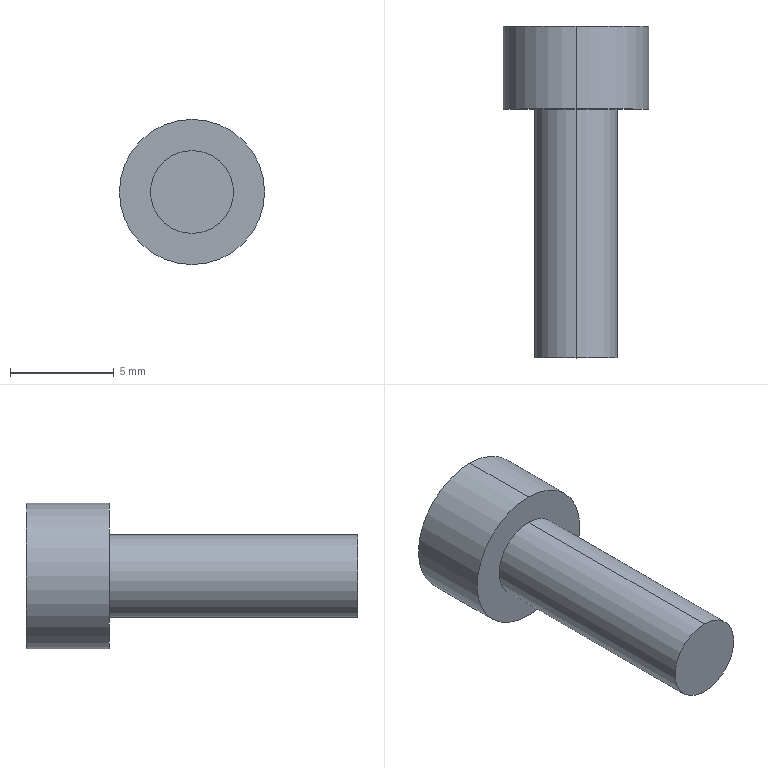Part | STEP file | NEZI-L_E-LMPJC30L35-14-15-LK5 | 1 solid | 14 faces | box 7 x 16 x 7 mm | volume 288.41 mm3 | plane 10 | cylinder 4 | commonest cylinder face diameters 4 x2 7 x2
STEP:
#1=CARTESIAN_POINT('',(0.,0.,0.));
#2=DIRECTION('',(0.,0.,1.));
#3=DIRECTION('',(1.,0.,0.));
#4=AXIS2_PLACEMENT_3D('',#1,#2,#3);
#5=CARTESIAN_POINT('',(0.,-12.,-2.));
#6=VERTEX_POINT('',#5);
#7=CARTESIAN_POINT('',(0.,-12.,2.));
#8=VERTEX_POINT('',#7);
#9=CARTESIAN_POINT('',(0.,-12.,0.));
#10=DIRECTION('',(0.,-1.,0.));
#11=DIRECTION('',(0.,0.,-1.));
#12=AXIS2_PLACEMENT_3D('',#9,#10,#11);
#13=CIRCLE('',#12,2.);
#14=CARTESIAN_POINT('',(0.,-12.,0.));
#15=DIRECTION('',(0.,1.,0.));
#16=DIRECTION('',(0.,0.,1.));
#17=AXIS2_PLACEMENT_3D('',#14,#15,#16);
#18=CYLINDRICAL_SURFACE('',#17,2.);
#19=CARTESIAN_POINT('',(3.142,0.));
#20=DIRECTION('',(-1.,0.));
#21=VECTOR('',#20,1.);
#22=LINE('',#19,#21);
#23=(GEOMETRIC_REPRESENTATION_CONTEXT(2)PARAMETRIC_REPRESENTATION_CONTEXT()REPRESENTATION_CONTEXT('',''));
#24=DEFINITIONAL_REPRESENTATION('',(#22),#23);
#25=PCURVE('',#18,#24);
#26=CARTESIAN_POINT('',(0.,-12.,0.));
#27=DIRECTION('',(0.,-1.,0.));
#28=DIRECTION('',(0.,0.,-1.));
#29=AXIS2_PLACEMENT_3D('',#26,#27,#28);
#30=PLANE('',#29);
#31=CARTESIAN_POINT('',(0.,0.));
#32=DIRECTION('',(1.,0.));
#33=AXIS2_PLACEMENT_2D('',#31,#32);
#34=CIRCLE('',#33,2.);
#35=(GEOMETRIC_REPRESENTATION_CONTEXT(2)PARAMETRIC_REPRESENTATION_CONTEXT()REPRESENTATION_CONTEXT('',''));
#36=DEFINITIONAL_REPRESENTATION('',(#34),#35);
#37=PCURVE('',#30,#36);
#38=SURFACE_CURVE('',#13,(#25,#37),.PCURVE_S1.);
#39=EDGE_CURVE('',#6,#8,#38,.T.);
#40=ORIENTED_EDGE('',*,*,#39,.F.);
#41=CARTESIAN_POINT('',(0.,0.,-2.));
#42=VERTEX_POINT('',#41);
#43=CARTESIAN_POINT('',(0.,-12.,-2.));
#44=DIRECTION('',(0.,1.,0.));
#45=VECTOR('',#44,1.);
#46=LINE('',#43,#45);
#47=CARTESIAN_POINT('',(3.142,0.));
#48=DIRECTION('',(0.,1.));
#49=VECTOR('',#48,1.);
#50=LINE('',#47,#49);
#51=(GEOMETRIC_REPRESENTATION_CONTEXT(2)PARAMETRIC_REPRESENTATION_CONTEXT()REPRESENTATION_CONTEXT('',''));
#52=DEFINITIONAL_REPRESENTATION('',(#50),#51);
#53=PCURVE('',#18,#52);
#54=CARTESIAN_POINT('',(0.,-12.,0.));
#55=DIRECTION('',(0.,1.,0.));
#56=DIRECTION('',(0.,0.,1.));
#57=AXIS2_PLACEMENT_3D('',#54,#55,#56);
#58=CYLINDRICAL_SURFACE('',#57,2.);
#59=CARTESIAN_POINT('',(3.142,0.));
#60=DIRECTION('',(0.,1.));
#61=VECTOR('',#60,1.);
#62=LINE('',#59,#61);
#63=(GEOMETRIC_REPRESENTATION_CONTEXT(2)PARAMETRIC_REPRESENTATION_CONTEXT()REPRESENTATION_CONTEXT('',''));
#64=DEFINITIONAL_REPRESENTATION('',(#62),#63);
#65=PCURVE('',#58,#64);
#66=SURFACE_CURVE('',#46,(#53,#65),.PCURVE_S1.);
#67=EDGE_CURVE('',#6,#42,#66,.T.);
#68=ORIENTED_EDGE('',*,*,#67,.T.);
#69=CARTESIAN_POINT('',(0.,0.,2.));
#70=VERTEX_POINT('',#69);
#71=CARTESIAN_POINT('',(0.,0.,0.));
#72=DIRECTION('',(0.,-1.,0.));
#73=DIRECTION('',(0.,0.,1.));
#74=AXIS2_PLACEMENT_3D('',#71,#72,#73);
#75=CIRCLE('',#74,2.);
#76=CARTESIAN_POINT('',(6.283,12.));
#77=DIRECTION('',(-1.,0.));
#78=VECTOR('',#77,1.);
#79=LINE('',#76,#78);
#80=(GEOMETRIC_REPRESENTATION_CONTEXT(2)PARAMETRIC_REPRESENTATION_CONTEXT()REPRESENTATION_CONTEXT('',''));
#81=DEFINITIONAL_REPRESENTATION('',(#79),#80);
#82=PCURVE('',#18,#81);
#83=CARTESIAN_POINT('',(0.,0.,0.));
#84=DIRECTION('',(0.,1.,0.));
#85=DIRECTION('',(0.,0.,1.));
#86=AXIS2_PLACEMENT_3D('',#83,#84,#85);
#87=PLANE('',#86);
#88=CARTESIAN_POINT('',(2.,0.));
#89=CARTESIAN_POINT('',(2.,-3.464));
#90=CARTESIAN_POINT('',(-1.,-1.732));
#91=CARTESIAN_POINT('',(-4.,0.));
#92=CARTESIAN_POINT('',(-1.,1.732));
#93=CARTESIAN_POINT('',(2.,3.464));
#94=CARTESIAN_POINT('',(2.,0.));
#95=(BOUNDED_CURVE()B_SPLINE_CURVE(2,(#88,#89,#90,#91,#92,#93,#94),.UNSPECIFIED.,.T.,.F.)B_SPLINE_CURVE_WITH_KNOTS((1,2,2,2,2,1),(-2.094,0.,2.094,4.189,6.283,8.378),.UNSPECIFIED.)CURVE()GEOMETRIC_REPRESENTATION_ITEM()RATIONAL_B_SPLINE_CURVE((1.,0.5,1.,0.5,1.,0.5,1.))REPRESENTATION_ITEM(''));
#96=(GEOMETRIC_REPRESENTATION_CONTEXT(2)PARAMETRIC_REPRESENTATION_CONTEXT()REPRESENTATION_CONTEXT('',''));
#97=DEFINITIONAL_REPRESENTATION('',(#95),#96);
#98=PCURVE('',#87,#97);
#99=SURFACE_CURVE('',#75,(#82,#98),.PCURVE_S1.);
#100=EDGE_CURVE('',#42,#70,#99,.T.);
#101=ORIENTED_EDGE('',*,*,#100,.T.);
#102=CARTESIAN_POINT('',(0.,-12.,2.));
#103=DIRECTION('',(0.,1.,0.));
#104=VECTOR('',#103,1.);
#105=LINE('',#102,#104);
#106=CARTESIAN_POINT('',(0.,0.));
#107=DIRECTION('',(0.,1.));
#108=VECTOR('',#107,1.);
#109=LINE('',#106,#108);
#110=(GEOMETRIC_REPRESENTATION_CONTEXT(2)PARAMETRIC_REPRESENTATION_CONTEXT()REPRESENTATION_CONTEXT('',''));
#111=DEFINITIONAL_REPRESENTATION('',(#109),#110);
#112=PCURVE('',#18,#111);
#113=CARTESIAN_POINT('',(6.283,0.));
#114=DIRECTION('',(0.,1.));
#115=VECTOR('',#114,1.);
#116=LINE('',#113,#115);
#117=(GEOMETRIC_REPRESENTATION_CONTEXT(2)PARAMETRIC_REPRESENTATION_CONTEXT()REPRESENTATION_CONTEXT('',''));
#118=DEFINITIONAL_REPRESENTATION('',(#116),#117);
#119=PCURVE('',#58,#118);
#120=SURFACE_CURVE('',#105,(#112,#119),.PCURVE_S1.);
#121=EDGE_CURVE('',#8,#70,#120,.T.);
#122=ORIENTED_EDGE('',*,*,#121,.F.);
#123=EDGE_LOOP('',(#40,#68,#101,#122));
#124=FACE_BOUND('',#123,.T.);
#125=ADVANCED_FACE('',(#124),#18,.T.);
#126=CARTESIAN_POINT('',(0.,4.,3.5));
#127=VERTEX_POINT('',#126);
#128=CARTESIAN_POINT('',(0.,4.,-3.5));
#129=VERTEX_POINT('',#128);
#130=CARTESIAN_POINT('',(0.,4.,0.));
#131=DIRECTION('',(0.,1.,0.));
#132=DIRECTION('',(0.,0.,1.));
#133=AXIS2_PLACEMENT_3D('',#130,#131,#132);
#134=CIRCLE('',#133,3.5);
#135=CARTESIAN_POINT('',(0.,4.,0.));
#136=DIRECTION('',(0.,-1.,0.));
#137=DIRECTION('',(0.,0.,-1.));
#138=AXIS2_PLACEMENT_3D('',#135,#136,#137);
#139=CYLINDRICAL_SURFACE('',#138,3.5);
#140=CARTESIAN_POINT('',(3.142,0.));
#141=DIRECTION('',(-1.,0.));
#142=VECTOR('',#141,1.);
#143=LINE('',#140,#142);
#144=(GEOMETRIC_REPRESENTATION_CONTEXT(2)PARAMETRIC_REPRESENTATION_CONTEXT()REPRESENTATION_CONTEXT('',''));
#145=DEFINITIONAL_REPRESENTATION('',(#143),#144);
#146=PCURVE('',#139,#145);
#147=CARTESIAN_POINT('',(0.,4.,0.));
#148=DIRECTION('',(0.,1.,0.));
#149=DIRECTION('',(0.,0.,1.));
#150=AXIS2_PLACEMENT_3D('',#147,#148,#149);
#151=PLANE('',#150);
#152=CARTESIAN_POINT('',(0.,0.));
#153=DIRECTION('',(1.,0.));
#154=AXIS2_PLACEMENT_2D('',#152,#153);
#155=CIRCLE('',#154,3.5);
#156=(GEOMETRIC_REPRESENTATION_CONTEXT(2)PARAMETRIC_REPRESENTATION_CONTEXT()REPRESENTATION_CONTEXT('',''));
#157=DEFINITIONAL_REPRESENTATION('',(#155),#156);
#158=PCURVE('',#151,#157);
#159=SURFACE_CURVE('',#134,(#146,#158),.PCURVE_S1.);
#160=EDGE_CURVE('',#127,#129,#159,.T.);
#161=ORIENTED_EDGE('',*,*,#160,.F.);
#162=CARTESIAN_POINT('',(0.,0.,3.5));
#163=VERTEX_POINT('',#162);
#164=CARTESIAN_POINT('',(0.,4.,3.5));
#165=DIRECTION('',(0.,-1.,0.));
#166=VECTOR('',#165,1.);
#167=LINE('',#164,#166);
#168=CARTESIAN_POINT('',(3.142,0.));
#169=DIRECTION('',(0.,1.));
#170=VECTOR('',#169,1.);
#171=LINE('',#168,#170);
#172=(GEOMETRIC_REPRESENTATION_CONTEXT(2)PARAMETRIC_REPRESENTATION_CONTEXT()REPRESENTATION_CONTEXT('',''));
#173=DEFINITIONAL_REPRESENTATION('',(#171),#172);
#174=PCURVE('',#139,#173);
#175=CARTESIAN_POINT('',(0.,4.,0.));
#176=DIRECTION('',(0.,-1.,0.));
#177=DIRECTION('',(0.,0.,-1.));
#178=AXIS2_PLACEMENT_3D('',#175,#176,#177);
#179=CYLINDRICAL_SURFACE('',#178,3.5);
#180=CARTESIAN_POINT('',(3.142,0.));
#181=DIRECTION('',(0.,1.));
#182=VECTOR('',#181,1.);
#183=LINE('',#180,#182);
#184=(GEOMETRIC_REPRESENTATION_CONTEXT(2)PARAMETRIC_REPRESENTATION_CONTEXT()REPRESENTATION_CONTEXT('',''));
#185=DEFINITIONAL_REPRESENTATION('',(#183),#184);
#186=PCURVE('',#179,#185);
#187=SURFACE_CURVE('',#167,(#174,#186),.PCURVE_S1.);
#188=EDGE_CURVE('',#127,#163,#187,.T.);
#189=ORIENTED_EDGE('',*,*,#188,.T.);
#190=CARTESIAN_POINT('',(0.,0.,-3.5));
#191=VERTEX_POINT('',#190);
#192=CARTESIAN_POINT('',(0.,0.,0.));
#193=DIRECTION('',(0.,1.,0.));
#194=DIRECTION('',(0.,0.,1.));
#195=AXIS2_PLACEMENT_3D('',#192,#193,#194);
#196=CIRCLE('',#195,3.5);
#197=CARTESIAN_POINT('',(3.142,4.));
#198=DIRECTION('',(-1.,0.));
#199=VECTOR('',#198,1.);
#200=LINE('',#197,#199);
#201=(GEOMETRIC_REPRESENTATION_CONTEXT(2)PARAMETRIC_REPRESENTATION_CONTEXT()REPRESENTATION_CONTEXT('',''));
#202=DEFINITIONAL_REPRESENTATION('',(#200),#201);
#203=PCURVE('',#139,#202);
#204=CARTESIAN_POINT('',(0.,0.));
#205=DIRECTION('',(1.,0.));
#206=AXIS2_PLACEMENT_2D('',#204,#205);
#207=CIRCLE('',#206,3.5);
#208=(GEOMETRIC_REPRESENTATION_CONTEXT(2)PARAMETRIC_REPRESENTATION_CONTEXT()REPRESENTATION_CONTEXT('',''));
#209=DEFINITIONAL_REPRESENTATION('',(#207),#208);
#210=PCURVE('',#87,#209);
#211=SURFACE_CURVE('',#196,(#203,#210),.PCURVE_S1.);
#212=EDGE_CURVE('',#163,#191,#211,.T.);
#213=ORIENTED_EDGE('',*,*,#212,.T.);
#214=CARTESIAN_POINT('',(0.,4.,-3.5));
#215=DIRECTION('',(0.,-1.,0.));
#216=VECTOR('',#215,1.);
#217=LINE('',#214,#216);
#218=CARTESIAN_POINT('',(0.,0.));
#219=DIRECTION('',(0.,1.));
#220=VECTOR('',#219,1.);
#221=LINE('',#218,#220);
#222=(GEOMETRIC_REPRESENTATION_CONTEXT(2)PARAMETRIC_REPRESENTATION_CONTEXT()REPRESENTATION_CONTEXT('',''));
#223=DEFINITIONAL_REPRESENTATION('',(#221),#222);
#224=PCURVE('',#139,#223);
#225=CARTESIAN_POINT('',(6.283,0.));
#226=DIRECTION('',(0.,1.));
#227=VECTOR('',#226,1.);
#228=LINE('',#225,#227);
#229=(GEOMETRIC_REPRESENTATION_CONTEXT(2)PARAMETRIC_REPRESENTATION_CONTEXT()REPRESENTATION_CONTEXT('',''));
#230=DEFINITIONAL_REPRESENTATION('',(#228),#229);
#231=PCURVE('',#179,#230);
#232=SURFACE_CURVE('',#217,(#224,#231),.PCURVE_S1.);
#233=EDGE_CURVE('',#129,#191,#232,.T.);
#234=ORIENTED_EDGE('',*,*,#233,.F.);
#235=EDGE_LOOP('',(#161,#189,#213,#234));
#236=FACE_BOUND('',#235,.T.);
#237=ADVANCED_FACE('',(#236),#139,.T.);
#238=ORIENTED_EDGE('',*,*,#188,.F.);
#239=CARTESIAN_POINT('',(0.,4.,0.));
#240=DIRECTION('',(0.,1.,0.));
#241=DIRECTION('',(0.,0.,1.));
#242=AXIS2_PLACEMENT_3D('',#239,#240,#241);
#243=CIRCLE('',#242,3.5);
#244=CARTESIAN_POINT('',(9.425,0.));
#245=DIRECTION('',(-1.,0.));
#246=VECTOR('',#245,1.);
#247=LINE('',#244,#246);
#248=(GEOMETRIC_REPRESENTATION_CONTEXT(2)PARAMETRIC_REPRESENTATION_CONTEXT()REPRESENTATION_CONTEXT('',''));
#249=DEFINITIONAL_REPRESENTATION('',(#247),#248);
#250=PCURVE('',#179,#249);
#251=CARTESIAN_POINT('',(0.,0.));
#252=DIRECTION('',(1.,0.));
#253=AXIS2_PLACEMENT_2D('',#251,#252);
#254=CIRCLE('',#253,3.5);
#255=(GEOMETRIC_REPRESENTATION_CONTEXT(2)PARAMETRIC_REPRESENTATION_CONTEXT()REPRESENTATION_CONTEXT('',''));
#256=DEFINITIONAL_REPRESENTATION('',(#254),#255);
#257=PCURVE('',#151,#256);
#258=SURFACE_CURVE('',#243,(#250,#257),.PCURVE_S1.);
#259=EDGE_CURVE('',#129,#127,#258,.T.);
#260=ORIENTED_EDGE('',*,*,#259,.F.);
#261=ORIENTED_EDGE('',*,*,#233,.T.);
#262=CARTESIAN_POINT('',(0.,0.,0.));
#263=DIRECTION('',(0.,1.,0.));
#264=DIRECTION('',(0.,0.,1.));
#265=AXIS2_PLACEMENT_3D('',#262,#263,#264);
#266=CIRCLE('',#265,3.5);
#267=CARTESIAN_POINT('',(9.425,4.));
#268=DIRECTION('',(-1.,0.));
#269=VECTOR('',#268,1.);
#270=LINE('',#267,#269);
#271=(GEOMETRIC_REPRESENTATION_CONTEXT(2)PARAMETRIC_REPRESENTATION_CONTEXT()REPRESENTATION_CONTEXT('',''));
#272=DEFINITIONAL_REPRESENTATION('',(#270),#271);
#273=PCURVE('',#179,#272);
#274=CARTESIAN_POINT('',(0.,0.));
#275=DIRECTION('',(1.,0.));
#276=AXIS2_PLACEMENT_2D('',#274,#275);
#277=CIRCLE('',#276,3.5);
#278=(GEOMETRIC_REPRESENTATION_CONTEXT(2)PARAMETRIC_REPRESENTATION_CONTEXT()REPRESENTATION_CONTEXT('',''));
#279=DEFINITIONAL_REPRESENTATION('',(#277),#278);
#280=PCURVE('',#87,#279);
#281=SURFACE_CURVE('',#266,(#273,#280),.PCURVE_S1.);
#282=EDGE_CURVE('',#191,#163,#281,.T.);
#283=ORIENTED_EDGE('',*,*,#282,.T.);
#284=EDGE_LOOP('',(#238,#260,#261,#283));
#285=FACE_BOUND('',#284,.T.);
#286=ADVANCED_FACE('',(#285),#179,.T.);
#287=CARTESIAN_POINT('',(1.535,4.,-0.8862));
#288=VERTEX_POINT('',#287);
#289=CARTESIAN_POINT('',(0.,4.,-1.772));
#290=VERTEX_POINT('',#289);
#291=CARTESIAN_POINT('',(1.535,4.,-0.8862));
#292=DIRECTION('',(-0.866,0.,-0.5));
#293=VECTOR('',#292,1.);
#294=LINE('',#291,#293);
#295=CARTESIAN_POINT('',(-0.8862,1.535));
#296=DIRECTION('',(-0.5,-0.866));
#297=VECTOR('',#296,1.);
#298=LINE('',#295,#297);
#299=(GEOMETRIC_REPRESENTATION_CONTEXT(2)PARAMETRIC_REPRESENTATION_CONTEXT()REPRESENTATION_CONTEXT('',''));
#300=DEFINITIONAL_REPRESENTATION('',(#298),#299);
#301=PCURVE('',#151,#300);
#302=CARTESIAN_POINT('',(1.535,2.,-0.8862));
#303=DIRECTION('',(0.5,0.,-0.866));
#304=DIRECTION('',(-0.866,0.,-0.5));
#305=AXIS2_PLACEMENT_3D('',#302,#303,#304);
#306=PLANE('',#305);
#307=CARTESIAN_POINT('',(0.,2.));
#308=DIRECTION('',(1.,0.));
#309=VECTOR('',#308,1.);
#310=LINE('',#307,#309);
#311=(GEOMETRIC_REPRESENTATION_CONTEXT(2)PARAMETRIC_REPRESENTATION_CONTEXT()REPRESENTATION_CONTEXT('',''));
#312=DEFINITIONAL_REPRESENTATION('',(#310),#311);
#313=PCURVE('',#306,#312);
#314=SURFACE_CURVE('',#294,(#301,#313),.PCURVE_S1.);
#315=EDGE_CURVE('',#288,#290,#314,.T.);
#316=ORIENTED_EDGE('',*,*,#315,.F.);
#317=CARTESIAN_POINT('',(1.535,4.,0.8862));
#318=VERTEX_POINT('',#317);
#319=CARTESIAN_POINT('',(1.535,4.,0.8862));
#320=DIRECTION('',(0.,0.,-1.));
#321=VECTOR('',#320,1.);
#322=LINE('',#319,#321);
#323=CARTESIAN_POINT('',(0.8862,1.535));
#324=DIRECTION('',(-1.,0.));
#325=VECTOR('',#324,1.);
#326=LINE('',#323,#325);
#327=(GEOMETRIC_REPRESENTATION_CONTEXT(2)PARAMETRIC_REPRESENTATION_CONTEXT()REPRESENTATION_CONTEXT('',''));
#328=DEFINITIONAL_REPRESENTATION('',(#326),#327);
#329=PCURVE('',#151,#328);
#330=CARTESIAN_POINT('',(1.535,2.,0.8862));
#331=DIRECTION('',(1.,0.,0.));
#332=DIRECTION('',(0.,0.,-1.));
#333=AXIS2_PLACEMENT_3D('',#330,#331,#332);
#334=PLANE('',#333);
#335=CARTESIAN_POINT('',(0.,2.));
#336=DIRECTION('',(1.,0.));
#337=VECTOR('',#336,1.);
#338=LINE('',#335,#337);
#339=(GEOMETRIC_REPRESENTATION_CONTEXT(2)PARAMETRIC_REPRESENTATION_CONTEXT()REPRESENTATION_CONTEXT('',''));
#340=DEFINITIONAL_REPRESENTATION('',(#338),#339);
#341=PCURVE('',#334,#340);
#342=SURFACE_CURVE('',#322,(#329,#341),.PCURVE_S1.);
#343=EDGE_CURVE('',#318,#288,#342,.T.);
#344=ORIENTED_EDGE('',*,*,#343,.F.);
#345=CARTESIAN_POINT('',(0.,4.,1.772));
#346=VERTEX_POINT('',#345);
#347=CARTESIAN_POINT('',(0.,4.,1.772));
#348=DIRECTION('',(0.866,0.,-0.5));
#349=VECTOR('',#348,1.);
#350=LINE('',#347,#349);
#351=CARTESIAN_POINT('',(1.772,0.));
#352=DIRECTION('',(-0.5,0.866));
#353=VECTOR('',#352,1.);
#354=LINE('',#351,#353);
#355=(GEOMETRIC_REPRESENTATION_CONTEXT(2)PARAMETRIC_REPRESENTATION_CONTEXT()REPRESENTATION_CONTEXT('',''));
#356=DEFINITIONAL_REPRESENTATION('',(#354),#355);
#357=PCURVE('',#151,#356);
#358=CARTESIAN_POINT('',(0.,2.,1.772));
#359=DIRECTION('',(0.5,0.,0.866));
#360=DIRECTION('',(0.866,0.,-0.5));
#361=AXIS2_PLACEMENT_3D('',#358,#359,#360);
#362=PLANE('',#361);
#363=CARTESIAN_POINT('',(0.,2.));
#364=DIRECTION('',(1.,0.));
#365=VECTOR('',#364,1.);
#366=LINE('',#363,#365);
#367=(GEOMETRIC_REPRESENTATION_CONTEXT(2)PARAMETRIC_REPRESENTATION_CONTEXT()REPRESENTATION_CONTEXT('',''));
#368=DEFINITIONAL_REPRESENTATION('',(#366),#367);
#369=PCURVE('',#362,#368);
#370=SURFACE_CURVE('',#350,(#357,#369),.PCURVE_S1.);
#371=EDGE_CURVE('',#346,#318,#370,.T.);
#372=ORIENTED_EDGE('',*,*,#371,.F.);
#373=CARTESIAN_POINT('',(-1.535,4.,0.8862));
#374=VERTEX_POINT('',#373);
#375=CARTESIAN_POINT('',(-1.535,4.,0.8862));
#376=DIRECTION('',(0.866,0.,0.5));
#377=VECTOR('',#376,1.);
#378=LINE('',#375,#377);
#379=CARTESIAN_POINT('',(0.8862,-1.535));
#380=DIRECTION('',(0.5,0.866));
#381=VECTOR('',#380,1.);
#382=LINE('',#379,#381);
#383=(GEOMETRIC_REPRESENTATION_CONTEXT(2)PARAMETRIC_REPRESENTATION_CONTEXT()REPRESENTATION_CONTEXT('',''));
#384=DEFINITIONAL_REPRESENTATION('',(#382),#383);
#385=PCURVE('',#151,#384);
#386=CARTESIAN_POINT('',(-1.535,2.,0.8862));
#387=DIRECTION('',(-0.5,0.,0.866));
#388=DIRECTION('',(0.866,0.,0.5));
#389=AXIS2_PLACEMENT_3D('',#386,#387,#388);
#390=PLANE('',#389);
#391=CARTESIAN_POINT('',(0.,2.));
#392=DIRECTION('',(1.,0.));
#393=VECTOR('',#392,1.);
#394=LINE('',#391,#393);
#395=(GEOMETRIC_REPRESENTATION_CONTEXT(2)PARAMETRIC_REPRESENTATION_CONTEXT()REPRESENTATION_CONTEXT('',''));
#396=DEFINITIONAL_REPRESENTATION('',(#394),#395);
#397=PCURVE('',#390,#396);
#398=SURFACE_CURVE('',#378,(#385,#397),.PCURVE_S1.);
#399=EDGE_CURVE('',#374,#346,#398,.T.);
#400=ORIENTED_EDGE('',*,*,#399,.F.);
#401=CARTESIAN_POINT('',(-1.535,4.,-0.8862));
#402=VERTEX_POINT('',#401);
#403=CARTESIAN_POINT('',(-1.535,4.,-0.8862));
#404=DIRECTION('',(0.,0.,1.));
#405=VECTOR('',#404,1.);
#406=LINE('',#403,#405);
#407=CARTESIAN_POINT('',(-0.8862,-1.535));
#408=DIRECTION('',(1.,0.));
#409=VECTOR('',#408,1.);
#410=LINE('',#407,#409);
#411=(GEOMETRIC_REPRESENTATION_CONTEXT(2)PARAMETRIC_REPRESENTATION_CONTEXT()REPRESENTATION_CONTEXT('',''));
#412=DEFINITIONAL_REPRESENTATION('',(#410),#411);
#413=PCURVE('',#151,#412);
#414=CARTESIAN_POINT('',(-1.535,2.,-0.8862));
#415=DIRECTION('',(-1.,0.,0.));
#416=DIRECTION('',(0.,0.,1.));
#417=AXIS2_PLACEMENT_3D('',#414,#415,#416);
#418=PLANE('',#417);
#419=CARTESIAN_POINT('',(0.,2.));
#420=DIRECTION('',(1.,0.));
#421=VECTOR('',#420,1.);
#422=LINE('',#419,#421);
#423=(GEOMETRIC_REPRESENTATION_CONTEXT(2)PARAMETRIC_REPRESENTATION_CONTEXT()REPRESENTATION_CONTEXT('',''));
#424=DEFINITIONAL_REPRESENTATION('',(#422),#423);
#425=PCURVE('',#418,#424);
#426=SURFACE_CURVE('',#406,(#413,#425),.PCURVE_S1.);
#427=EDGE_CURVE('',#402,#374,#426,.T.);
#428=ORIENTED_EDGE('',*,*,#427,.F.);
#429=CARTESIAN_POINT('',(0.,4.,-1.772));
#430=DIRECTION('',(-0.866,0.,0.5));
#431=VECTOR('',#430,1.);
#432=LINE('',#429,#431);
#433=CARTESIAN_POINT('',(-1.772,0.));
#434=DIRECTION('',(0.5,-0.866));
#435=VECTOR('',#434,1.);
#436=LINE('',#433,#435);
#437=(GEOMETRIC_REPRESENTATION_CONTEXT(2)PARAMETRIC_REPRESENTATION_CONTEXT()REPRESENTATION_CONTEXT('',''));
#438=DEFINITIONAL_REPRESENTATION('',(#436),#437);
#439=PCURVE('',#151,#438);
#440=CARTESIAN_POINT('',(0.,2.,-1.772));
#441=DIRECTION('',(-0.5,0.,-0.866));
#442=DIRECTION('',(-0.866,0.,0.5));
#443=AXIS2_PLACEMENT_3D('',#440,#441,#442);
#444=PLANE('',#443);
#445=CARTESIAN_POINT('',(0.,2.));
#446=DIRECTION('',(1.,0.));
#447=VECTOR('',#446,1.);
#448=LINE('',#445,#447);
#449=(GEOMETRIC_REPRESENTATION_CONTEXT(2)PARAMETRIC_REPRESENTATION_CONTEXT()REPRESENTATION_CONTEXT('',''));
#450=DEFINITIONAL_REPRESENTATION('',(#448),#449);
#451=PCURVE('',#444,#450);
#452=SURFACE_CURVE('',#432,(#439,#451),.PCURVE_S1.);
#453=EDGE_CURVE('',#290,#402,#452,.T.);
#454=ORIENTED_EDGE('',*,*,#453,.F.);
#455=EDGE_LOOP('',(#316,#344,#372,#400,#428,#454));
#456=FACE_BOUND('',#455,.T.);
#457=ORIENTED_EDGE('',*,*,#259,.T.);
#458=ORIENTED_EDGE('',*,*,#160,.T.);
#459=EDGE_LOOP('',(#457,#458));
#460=FACE_BOUND('',#459,.T.);
#461=ADVANCED_FACE('',(#456,#460),#151,.T.);
#462=CARTESIAN_POINT('',(0.,0.,0.));
#463=DIRECTION('',(0.,-1.,0.));
#464=DIRECTION('',(0.,0.,1.));
#465=AXIS2_PLACEMENT_3D('',#462,#463,#464);
#466=CIRCLE('',#465,2.);
#467=CARTESIAN_POINT('',(2.,0.));
#468=CARTESIAN_POINT('',(2.,-3.464));
#469=CARTESIAN_POINT('',(-1.,-1.732));
#470=CARTESIAN_POINT('',(-4.,0.));
#471=CARTESIAN_POINT('',(-1.,1.732));
#472=CARTESIAN_POINT('',(2.,3.464));
#473=CARTESIAN_POINT('',(2.,0.));
#474=(BOUNDED_CURVE()B_SPLINE_CURVE(2,(#467,#468,#469,#470,#471,#472,#473),.UNSPECIFIED.,.T.,.F.)B_SPLINE_CURVE_WITH_KNOTS((1,2,2,2,2,1),(-2.094,0.,2.094,4.189,6.283,8.378),.UNSPECIFIED.)CURVE()GEOMETRIC_REPRESENTATION_ITEM()RATIONAL_B_SPLINE_CURVE((1.,0.5,1.,0.5,1.,0.5,1.))REPRESENTATION_ITEM(''));
#475=(GEOMETRIC_REPRESENTATION_CONTEXT(2)PARAMETRIC_REPRESENTATION_CONTEXT()REPRESENTATION_CONTEXT('',''));
#476=DEFINITIONAL_REPRESENTATION('',(#474),#475);
#477=PCURVE('',#87,#476);
#478=CARTESIAN_POINT('',(6.283,12.));
#479=DIRECTION('',(-1.,0.));
#480=VECTOR('',#479,1.);
#481=LINE('',#478,#480);
#482=(GEOMETRIC_REPRESENTATION_CONTEXT(2)PARAMETRIC_REPRESENTATION_CONTEXT()REPRESENTATION_CONTEXT('',''));
#483=DEFINITIONAL_REPRESENTATION('',(#481),#482);
#484=PCURVE('',#58,#483);
#485=SURFACE_CURVE('',#466,(#477,#484),.PCURVE_S1.);
#486=EDGE_CURVE('',#70,#42,#485,.T.);
#487=ORIENTED_EDGE('',*,*,#486,.F.);
#488=ORIENTED_EDGE('',*,*,#100,.F.);
#489=EDGE_LOOP('',(#487,#488));
#490=FACE_BOUND('',#489,.T.);
#491=ORIENTED_EDGE('',*,*,#282,.F.);
#492=ORIENTED_EDGE('',*,*,#212,.F.);
#493=EDGE_LOOP('',(#491,#492));
#494=FACE_BOUND('',#493,.T.);
#495=ADVANCED_FACE('',(#490,#494),#87,.F.);
#496=ORIENTED_EDGE('',*,*,#67,.F.);
#497=CARTESIAN_POINT('',(0.,-12.,0.));
#498=DIRECTION('',(0.,-1.,0.));
#499=DIRECTION('',(0.,0.,-1.));
#500=AXIS2_PLACEMENT_3D('',#497,#498,#499);
#501=CIRCLE('',#500,2.);
#502=CARTESIAN_POINT('',(9.425,0.));
#503=DIRECTION('',(-1.,0.));
#504=VECTOR('',#503,1.);
#505=LINE('',#502,#504);
#506=(GEOMETRIC_REPRESENTATION_CONTEXT(2)PARAMETRIC_REPRESENTATION_CONTEXT()REPRESENTATION_CONTEXT('',''));
#507=DEFINITIONAL_REPRESENTATION('',(#505),#506);
#508=PCURVE('',#58,#507);
#509=CARTESIAN_POINT('',(0.,0.));
#510=DIRECTION('',(1.,0.));
#511=AXIS2_PLACEMENT_2D('',#509,#510);
#512=CIRCLE('',#511,2.);
#513=(GEOMETRIC_REPRESENTATION_CONTEXT(2)PARAMETRIC_REPRESENTATION_CONTEXT()REPRESENTATION_CONTEXT('',''));
#514=DEFINITIONAL_REPRESENTATION('',(#512),#513);
#515=PCURVE('',#30,#514);
#516=SURFACE_CURVE('',#501,(#508,#515),.PCURVE_S1.);
#517=EDGE_CURVE('',#8,#6,#516,.T.);
#518=ORIENTED_EDGE('',*,*,#517,.F.);
#519=ORIENTED_EDGE('',*,*,#121,.T.);
#520=ORIENTED_EDGE('',*,*,#486,.T.);
#521=EDGE_LOOP('',(#496,#518,#519,#520));
#522=FACE_BOUND('',#521,.T.);
#523=ADVANCED_FACE('',(#522),#58,.T.);
#524=ORIENTED_EDGE('',*,*,#517,.T.);
#525=ORIENTED_EDGE('',*,*,#39,.T.);
#526=EDGE_LOOP('',(#524,#525));
#527=FACE_BOUND('',#526,.T.);
#528=ADVANCED_FACE('',(#527),#30,.T.);
#529=ORIENTED_EDGE('',*,*,#315,.T.);
#530=CARTESIAN_POINT('',(0.,2.,-1.772));
#531=VERTEX_POINT('',#530);
#532=CARTESIAN_POINT('',(0.,2.,-1.772));
#533=DIRECTION('',(0.,1.,0.));
#534=VECTOR('',#533,1.);
#535=LINE('',#532,#534);
#536=CARTESIAN_POINT('',(1.772,0.));
#537=DIRECTION('',(0.,1.));
#538=VECTOR('',#537,1.);
#539=LINE('',#536,#538);
#540=(GEOMETRIC_REPRESENTATION_CONTEXT(2)PARAMETRIC_REPRESENTATION_CONTEXT()REPRESENTATION_CONTEXT('',''));
#541=DEFINITIONAL_REPRESENTATION('',(#539),#540);
#542=PCURVE('',#306,#541);
#543=CARTESIAN_POINT('',(0.,0.));
#544=DIRECTION('',(0.,1.));
#545=VECTOR('',#544,1.);
#546=LINE('',#543,#545);
#547=(GEOMETRIC_REPRESENTATION_CONTEXT(2)PARAMETRIC_REPRESENTATION_CONTEXT()REPRESENTATION_CONTEXT('',''));
#548=DEFINITIONAL_REPRESENTATION('',(#546),#547);
#549=PCURVE('',#444,#548);
#550=SURFACE_CURVE('',#535,(#542,#549),.PCURVE_S1.);
#551=EDGE_CURVE('',#531,#290,#550,.T.);
#552=ORIENTED_EDGE('',*,*,#551,.F.);
#553=CARTESIAN_POINT('',(1.535,2.,-0.8862));
#554=VERTEX_POINT('',#553);
#555=CARTESIAN_POINT('',(1.535,2.,-0.8862));
#556=DIRECTION('',(-0.866,0.,-0.5));
#557=VECTOR('',#556,1.);
#558=LINE('',#555,#557);
#559=CARTESIAN_POINT('',(0.,0.));
#560=DIRECTION('',(1.,0.));
#561=VECTOR('',#560,1.);
#562=LINE('',#559,#561);
#563=(GEOMETRIC_REPRESENTATION_CONTEXT(2)PARAMETRIC_REPRESENTATION_CONTEXT()REPRESENTATION_CONTEXT('',''));
#564=DEFINITIONAL_REPRESENTATION('',(#562),#563);
#565=PCURVE('',#306,#564);
#566=CARTESIAN_POINT('',(0.,2.,0.));
#567=DIRECTION('',(0.,1.,0.));
#568=DIRECTION('',(0.,0.,1.));
#569=AXIS2_PLACEMENT_3D('',#566,#567,#568);
#570=PLANE('',#569);
#571=CARTESIAN_POINT('',(-0.8862,1.535));
#572=DIRECTION('',(-0.5,-0.866));
#573=VECTOR('',#572,1.);
#574=LINE('',#571,#573);
#575=(GEOMETRIC_REPRESENTATION_CONTEXT(2)PARAMETRIC_REPRESENTATION_CONTEXT()REPRESENTATION_CONTEXT('',''));
#576=DEFINITIONAL_REPRESENTATION('',(#574),#575);
#577=PCURVE('',#570,#576);
#578=SURFACE_CURVE('',#558,(#565,#577),.PCURVE_S1.);
#579=EDGE_CURVE('',#554,#531,#578,.T.);
#580=ORIENTED_EDGE('',*,*,#579,.F.);
#581=CARTESIAN_POINT('',(1.535,2.,-0.8862));
#582=DIRECTION('',(0.,1.,0.));
#583=VECTOR('',#582,1.);
#584=LINE('',#581,#583);
#585=CARTESIAN_POINT('',(0.,0.));
#586=DIRECTION('',(0.,1.));
#587=VECTOR('',#586,1.);
#588=LINE('',#585,#587);
#589=(GEOMETRIC_REPRESENTATION_CONTEXT(2)PARAMETRIC_REPRESENTATION_CONTEXT()REPRESENTATION_CONTEXT('',''));
#590=DEFINITIONAL_REPRESENTATION('',(#588),#589);
#591=PCURVE('',#306,#590);
#592=CARTESIAN_POINT('',(1.772,0.));
#593=DIRECTION('',(0.,1.));
#594=VECTOR('',#593,1.);
#595=LINE('',#592,#594);
#596=(GEOMETRIC_REPRESENTATION_CONTEXT(2)PARAMETRIC_REPRESENTATION_CONTEXT()REPRESENTATION_CONTEXT('',''));
#597=DEFINITIONAL_REPRESENTATION('',(#595),#596);
#598=PCURVE('',#334,#597);
#599=SURFACE_CURVE('',#584,(#591,#598),.PCURVE_S1.);
#600=EDGE_CURVE('',#554,#288,#599,.T.);
#601=ORIENTED_EDGE('',*,*,#600,.T.);
#602=EDGE_LOOP('',(#529,#552,#580,#601));
#603=FACE_BOUND('',#602,.T.);
#604=ADVANCED_FACE('',(#603),#306,.F.);
#605=ORIENTED_EDGE('',*,*,#343,.T.);
#606=ORIENTED_EDGE('',*,*,#600,.F.);
#607=CARTESIAN_POINT('',(1.535,2.,0.8862));
#608=VERTEX_POINT('',#607);
#609=CARTESIAN_POINT('',(1.535,2.,0.8862));
#610=DIRECTION('',(0.,0.,-1.));
#611=VECTOR('',#610,1.);
#612=LINE('',#609,#611);
#613=CARTESIAN_POINT('',(0.,0.));
#614=DIRECTION('',(1.,0.));
#615=VECTOR('',#614,1.);
#616=LINE('',#613,#615);
#617=(GEOMETRIC_REPRESENTATION_CONTEXT(2)PARAMETRIC_REPRESENTATION_CONTEXT()REPRESENTATION_CONTEXT('',''));
#618=DEFINITIONAL_REPRESENTATION('',(#616),#617);
#619=PCURVE('',#334,#618);
#620=CARTESIAN_POINT('',(0.8862,1.535));
#621=DIRECTION('',(-1.,0.));
#622=VECTOR('',#621,1.);
#623=LINE('',#620,#622);
#624=(GEOMETRIC_REPRESENTATION_CONTEXT(2)PARAMETRIC_REPRESENTATION_CONTEXT()REPRESENTATION_CONTEXT('',''));
#625=DEFINITIONAL_REPRESENTATION('',(#623),#624);
#626=PCURVE('',#570,#625);
#627=SURFACE_CURVE('',#612,(#619,#626),.PCURVE_S1.);
#628=EDGE_CURVE('',#608,#554,#627,.T.);
#629=ORIENTED_EDGE('',*,*,#628,.F.);
#630=CARTESIAN_POINT('',(1.535,2.,0.8862));
#631=DIRECTION('',(0.,1.,0.));
#632=VECTOR('',#631,1.);
#633=LINE('',#630,#632);
#634=CARTESIAN_POINT('',(0.,0.));
#635=DIRECTION('',(0.,1.));
#636=VECTOR('',#635,1.);
#637=LINE('',#634,#636);
#638=(GEOMETRIC_REPRESENTATION_CONTEXT(2)PARAMETRIC_REPRESENTATION_CONTEXT()REPRESENTATION_CONTEXT('',''));
#639=DEFINITIONAL_REPRESENTATION('',(#637),#638);
#640=PCURVE('',#334,#639);
#641=CARTESIAN_POINT('',(1.772,0.));
#642=DIRECTION('',(0.,1.));
#643=VECTOR('',#642,1.);
#644=LINE('',#641,#643);
#645=(GEOMETRIC_REPRESENTATION_CONTEXT(2)PARAMETRIC_REPRESENTATION_CONTEXT()REPRESENTATION_CONTEXT('',''));
#646=DEFINITIONAL_REPRESENTATION('',(#644),#645);
#647=PCURVE('',#362,#646);
#648=SURFACE_CURVE('',#633,(#640,#647),.PCURVE_S1.);
#649=EDGE_CURVE('',#608,#318,#648,.T.);
#650=ORIENTED_EDGE('',*,*,#649,.T.);
#651=EDGE_LOOP('',(#605,#606,#629,#650));
#652=FACE_BOUND('',#651,.T.);
#653=ADVANCED_FACE('',(#652),#334,.F.);
#654=ORIENTED_EDGE('',*,*,#371,.T.);
#655=ORIENTED_EDGE('',*,*,#649,.F.);
#656=CARTESIAN_POINT('',(0.,2.,1.772));
#657=VERTEX_POINT('',#656);
#658=CARTESIAN_POINT('',(0.,2.,1.772));
#659=DIRECTION('',(0.866,0.,-0.5));
#660=VECTOR('',#659,1.);
#661=LINE('',#658,#660);
#662=CARTESIAN_POINT('',(0.,0.));
#663=DIRECTION('',(1.,0.));
#664=VECTOR('',#663,1.);
#665=LINE('',#662,#664);
#666=(GEOMETRIC_REPRESENTATION_CONTEXT(2)PARAMETRIC_REPRESENTATION_CONTEXT()REPRESENTATION_CONTEXT('',''));
#667=DEFINITIONAL_REPRESENTATION('',(#665),#666);
#668=PCURVE('',#362,#667);
#669=CARTESIAN_POINT('',(1.772,0.));
#670=DIRECTION('',(-0.5,0.866));
#671=VECTOR('',#670,1.);
#672=LINE('',#669,#671);
#673=(GEOMETRIC_REPRESENTATION_CONTEXT(2)PARAMETRIC_REPRESENTATION_CONTEXT()REPRESENTATION_CONTEXT('',''));
#674=DEFINITIONAL_REPRESENTATION('',(#672),#673);
#675=PCURVE('',#570,#674);
#676=SURFACE_CURVE('',#661,(#668,#675),.PCURVE_S1.);
#677=EDGE_CURVE('',#657,#608,#676,.T.);
#678=ORIENTED_EDGE('',*,*,#677,.F.);
#679=CARTESIAN_POINT('',(0.,2.,1.772));
#680=DIRECTION('',(0.,1.,0.));
#681=VECTOR('',#680,1.);
#682=LINE('',#679,#681);
#683=CARTESIAN_POINT('',(0.,0.));
#684=DIRECTION('',(0.,1.));
#685=VECTOR('',#684,1.);
#686=LINE('',#683,#685);
#687=(GEOMETRIC_REPRESENTATION_CONTEXT(2)PARAMETRIC_REPRESENTATION_CONTEXT()REPRESENTATION_CONTEXT('',''));
#688=DEFINITIONAL_REPRESENTATION('',(#686),#687);
#689=PCURVE('',#362,#688);
#690=CARTESIAN_POINT('',(1.772,0.));
#691=DIRECTION('',(0.,1.));
#692=VECTOR('',#691,1.);
#693=LINE('',#690,#692);
#694=(GEOMETRIC_REPRESENTATION_CONTEXT(2)PARAMETRIC_REPRESENTATION_CONTEXT()REPRESENTATION_CONTEXT('',''));
#695=DEFINITIONAL_REPRESENTATION('',(#693),#694);
#696=PCURVE('',#390,#695);
#697=SURFACE_CURVE('',#682,(#689,#696),.PCURVE_S1.);
#698=EDGE_CURVE('',#657,#346,#697,.T.);
#699=ORIENTED_EDGE('',*,*,#698,.T.);
#700=EDGE_LOOP('',(#654,#655,#678,#699));
#701=FACE_BOUND('',#700,.T.);
#702=ADVANCED_FACE('',(#701),#362,.F.);
#703=ORIENTED_EDGE('',*,*,#399,.T.);
#704=ORIENTED_EDGE('',*,*,#698,.F.);
#705=CARTESIAN_POINT('',(-1.535,2.,0.8862));
#706=VERTEX_POINT('',#705);
#707=CARTESIAN_POINT('',(-1.535,2.,0.8862));
#708=DIRECTION('',(0.866,0.,0.5));
#709=VECTOR('',#708,1.);
#710=LINE('',#707,#709);
#711=CARTESIAN_POINT('',(0.,0.));
#712=DIRECTION('',(1.,0.));
#713=VECTOR('',#712,1.);
#714=LINE('',#711,#713);
#715=(GEOMETRIC_REPRESENTATION_CONTEXT(2)PARAMETRIC_REPRESENTATION_CONTEXT()REPRESENTATION_CONTEXT('',''));
#716=DEFINITIONAL_REPRESENTATION('',(#714),#715);
#717=PCURVE('',#390,#716);
#718=CARTESIAN_POINT('',(0.8862,-1.535));
#719=DIRECTION('',(0.5,0.866));
#720=VECTOR('',#719,1.);
#721=LINE('',#718,#720);
#722=(GEOMETRIC_REPRESENTATION_CONTEXT(2)PARAMETRIC_REPRESENTATION_CONTEXT()REPRESENTATION_CONTEXT('',''));
#723=DEFINITIONAL_REPRESENTATION('',(#721),#722);
#724=PCURVE('',#570,#723);
#725=SURFACE_CURVE('',#710,(#717,#724),.PCURVE_S1.);
#726=EDGE_CURVE('',#706,#657,#725,.T.);
#727=ORIENTED_EDGE('',*,*,#726,.F.);
#728=CARTESIAN_POINT('',(-1.535,2.,0.8862));
#729=DIRECTION('',(0.,1.,0.));
#730=VECTOR('',#729,1.);
#731=LINE('',#728,#730);
#732=CARTESIAN_POINT('',(0.,0.));
#733=DIRECTION('',(0.,1.));
#734=VECTOR('',#733,1.);
#735=LINE('',#732,#734);
#736=(GEOMETRIC_REPRESENTATION_CONTEXT(2)PARAMETRIC_REPRESENTATION_CONTEXT()REPRESENTATION_CONTEXT('',''));
#737=DEFINITIONAL_REPRESENTATION('',(#735),#736);
#738=PCURVE('',#390,#737);
#739=CARTESIAN_POINT('',(1.772,0.));
#740=DIRECTION('',(0.,1.));
#741=VECTOR('',#740,1.);
#742=LINE('',#739,#741);
#743=(GEOMETRIC_REPRESENTATION_CONTEXT(2)PARAMETRIC_REPRESENTATION_CONTEXT()REPRESENTATION_CONTEXT('',''));
#744=DEFINITIONAL_REPRESENTATION('',(#742),#743);
#745=PCURVE('',#418,#744);
#746=SURFACE_CURVE('',#731,(#738,#745),.PCURVE_S1.);
#747=EDGE_CURVE('',#706,#374,#746,.T.);
#748=ORIENTED_EDGE('',*,*,#747,.T.);
#749=EDGE_LOOP('',(#703,#704,#727,#748));
#750=FACE_BOUND('',#749,.T.);
#751=ADVANCED_FACE('',(#750),#390,.F.);
#752=ORIENTED_EDGE('',*,*,#427,.T.);
#753=ORIENTED_EDGE('',*,*,#747,.F.);
#754=CARTESIAN_POINT('',(-1.535,2.,-0.8862));
#755=VERTEX_POINT('',#754);
#756=CARTESIAN_POINT('',(-1.535,2.,-0.8862));
#757=DIRECTION('',(0.,0.,1.));
#758=VECTOR('',#757,1.);
#759=LINE('',#756,#758);
#760=CARTESIAN_POINT('',(0.,0.));
#761=DIRECTION('',(1.,0.));
#762=VECTOR('',#761,1.);
#763=LINE('',#760,#762);
#764=(GEOMETRIC_REPRESENTATION_CONTEXT(2)PARAMETRIC_REPRESENTATION_CONTEXT()REPRESENTATION_CONTEXT('',''));
#765=DEFINITIONAL_REPRESENTATION('',(#763),#764);
#766=PCURVE('',#418,#765);
#767=CARTESIAN_POINT('',(-0.8862,-1.535));
#768=DIRECTION('',(1.,0.));
#769=VECTOR('',#768,1.);
#770=LINE('',#767,#769);
#771=(GEOMETRIC_REPRESENTATION_CONTEXT(2)PARAMETRIC_REPRESENTATION_CONTEXT()REPRESENTATION_CONTEXT('',''));
#772=DEFINITIONAL_REPRESENTATION('',(#770),#771);
#773=PCURVE('',#570,#772);
#774=SURFACE_CURVE('',#759,(#766,#773),.PCURVE_S1.);
#775=EDGE_CURVE('',#755,#706,#774,.T.);
#776=ORIENTED_EDGE('',*,*,#775,.F.);
#777=CARTESIAN_POINT('',(-1.535,2.,-0.8862));
#778=DIRECTION('',(0.,1.,0.));
#779=VECTOR('',#778,1.);
#780=LINE('',#777,#779);
#781=CARTESIAN_POINT('',(0.,0.));
#782=DIRECTION('',(0.,1.));
#783=VECTOR('',#782,1.);
#784=LINE('',#781,#783);
#785=(GEOMETRIC_REPRESENTATION_CONTEXT(2)PARAMETRIC_REPRESENTATION_CONTEXT()REPRESENTATION_CONTEXT('',''));
#786=DEFINITIONAL_REPRESENTATION('',(#784),#785);
#787=PCURVE('',#418,#786);
#788=CARTESIAN_POINT('',(1.772,0.));
#789=DIRECTION('',(0.,1.));
#790=VECTOR('',#789,1.);
#791=LINE('',#788,#790);
#792=(GEOMETRIC_REPRESENTATION_CONTEXT(2)PARAMETRIC_REPRESENTATION_CONTEXT()REPRESENTATION_CONTEXT('',''));
#793=DEFINITIONAL_REPRESENTATION('',(#791),#792);
#794=PCURVE('',#444,#793);
#795=SURFACE_CURVE('',#780,(#787,#794),.PCURVE_S1.);
#796=EDGE_CURVE('',#755,#402,#795,.T.);
#797=ORIENTED_EDGE('',*,*,#796,.T.);
#798=EDGE_LOOP('',(#752,#753,#776,#797));
#799=FACE_BOUND('',#798,.T.);
#800=ADVANCED_FACE('',(#799),#418,.F.);
#801=ORIENTED_EDGE('',*,*,#453,.T.);
#802=ORIENTED_EDGE('',*,*,#796,.F.);
#803=CARTESIAN_POINT('',(0.,2.,-1.772));
#804=DIRECTION('',(-0.866,0.,0.5));
#805=VECTOR('',#804,1.);
#806=LINE('',#803,#805);
#807=CARTESIAN_POINT('',(0.,0.));
#808=DIRECTION('',(1.,0.));
#809=VECTOR('',#808,1.);
#810=LINE('',#807,#809);
#811=(GEOMETRIC_REPRESENTATION_CONTEXT(2)PARAMETRIC_REPRESENTATION_CONTEXT()REPRESENTATION_CONTEXT('',''));
#812=DEFINITIONAL_REPRESENTATION('',(#810),#811);
#813=PCURVE('',#444,#812);
#814=CARTESIAN_POINT('',(-1.772,0.));
#815=DIRECTION('',(0.5,-0.866));
#816=VECTOR('',#815,1.);
#817=LINE('',#814,#816);
#818=(GEOMETRIC_REPRESENTATION_CONTEXT(2)PARAMETRIC_REPRESENTATION_CONTEXT()REPRESENTATION_CONTEXT('',''));
#819=DEFINITIONAL_REPRESENTATION('',(#817),#818);
#820=PCURVE('',#570,#819);
#821=SURFACE_CURVE('',#806,(#813,#820),.PCURVE_S1.);
#822=EDGE_CURVE('',#531,#755,#821,.T.);
#823=ORIENTED_EDGE('',*,*,#822,.F.);
#824=ORIENTED_EDGE('',*,*,#551,.T.);
#825=EDGE_LOOP('',(#801,#802,#823,#824));
#826=FACE_BOUND('',#825,.T.);
#827=ADVANCED_FACE('',(#826),#444,.F.);
#828=ORIENTED_EDGE('',*,*,#579,.T.);
#829=ORIENTED_EDGE('',*,*,#822,.T.);
#830=ORIENTED_EDGE('',*,*,#775,.T.);
#831=ORIENTED_EDGE('',*,*,#726,.T.);
#832=ORIENTED_EDGE('',*,*,#677,.T.);
#833=ORIENTED_EDGE('',*,*,#628,.T.);
#834=EDGE_LOOP('',(#828,#829,#830,#831,#832,#833));
#835=FACE_BOUND('',#834,.T.);
#836=ADVANCED_FACE('',(#835),#570,.T.);
#837=CLOSED_SHELL('',(#125,#237,#286,#461,#495,#523,#528,#604,#653,#702,#751,#800,#827,#836));
#838=MANIFOLD_SOLID_BREP('',#837);
#839=(LENGTH_UNIT()NAMED_UNIT(*)SI_UNIT(.MILLI.,.METRE.));
#840=UNCERTAINTY_MEASURE_WITH_UNIT(LENGTH_MEASURE(0.0000001),#839,'','');
#841=(NAMED_UNIT(*)PLANE_ANGLE_UNIT()SI_UNIT($,.RADIAN.));
#842=(NAMED_UNIT(*)SI_UNIT($,.STERADIAN.)SOLID_ANGLE_UNIT());
#843=(GEOMETRIC_REPRESENTATION_CONTEXT(3)GLOBAL_UNCERTAINTY_ASSIGNED_CONTEXT((#840))GLOBAL_UNIT_ASSIGNED_CONTEXT((#839,#841,#842))REPRESENTATION_CONTEXT('',''));
#844=ADVANCED_BREP_SHAPE_REPRESENTATION('',(#4,#838),#843);